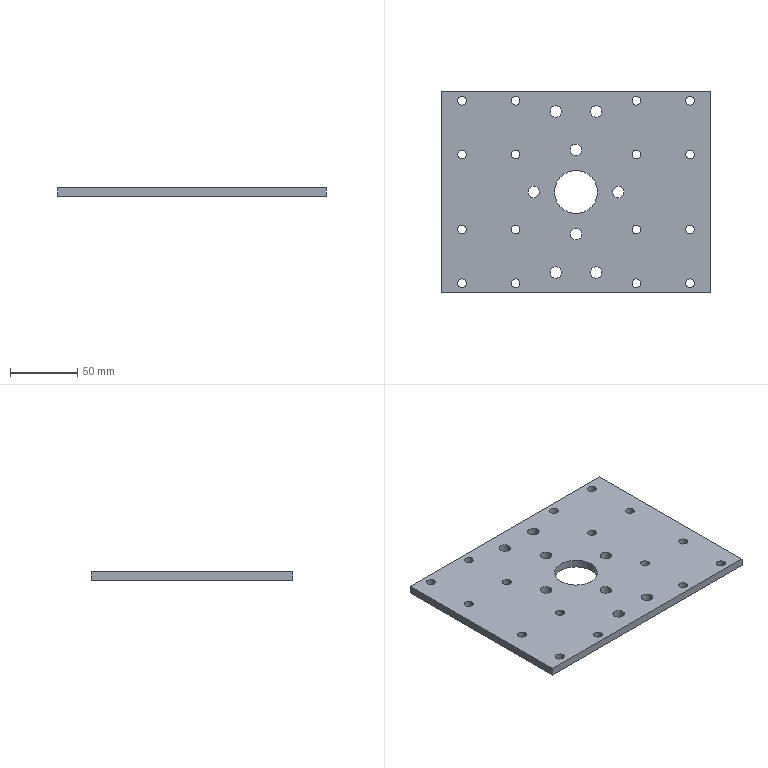Part | STEP file | 20312 | 1 solid | 56 faces | box 200 x 150 x 6 mm | volume 169265 mm3 | cylinder 50 | plane 6 | commonest cylinder face diameters 6.5 x32 8.5 x16 32 x2